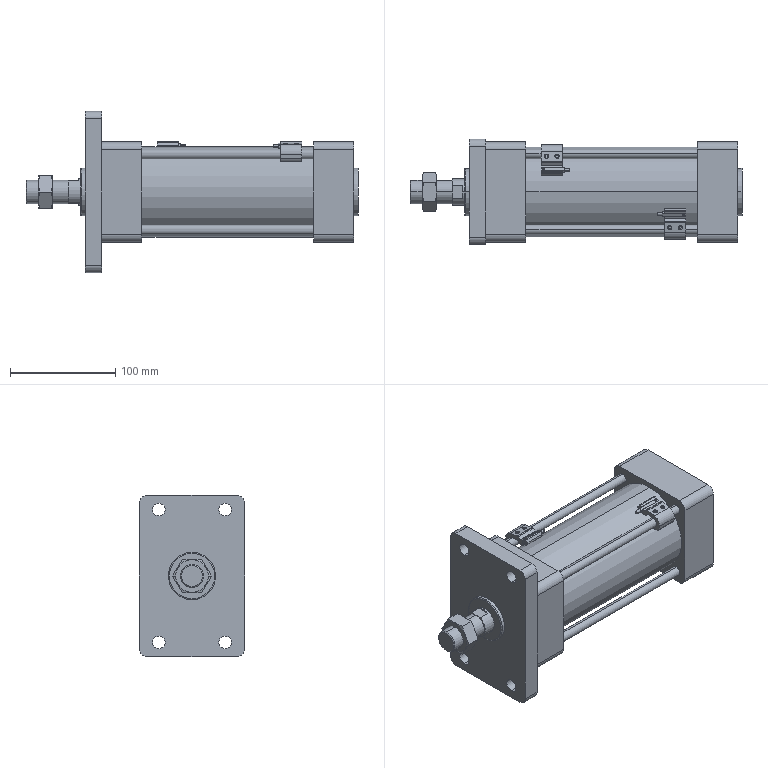Part | SolidWorks | features BaseBody 8 | 8 solids | 384 faces | box 315 x 100 x 153 mm | volume 1372991 mm3 | plane 193 | cylinder 155 | cone 34 | spline 2 | commonest cylinder face diameters 12 x27 4 x22 8.376 x16 11 x16 2 x9 9 x8